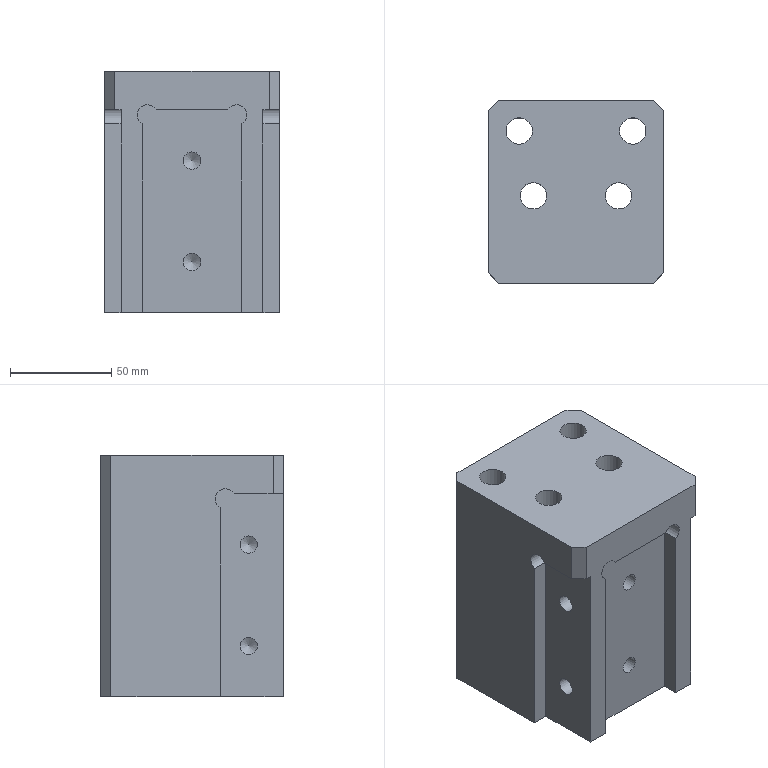Part | NX | features UB-5 2 | 1 solid | 50 faces | box 86 x 90 x 119 mm | volume 701688 mm3 | plane 24 | cylinder 19 | cone 7 | commonest cylinder face diameters 8.5 x6 10 x4 13.007 x4 20 x4 8.506 x1
STEP:
#1=CARTESIAN_POINT('',(3162.594,-722.122,881.466));
#2=VERTEX_POINT('',#1);
#3=CARTESIAN_POINT('',(3162.594,-722.122,885.716));
#4=DIRECTION('',(0.,1.,0.));
#5=DIRECTION('',(0.,0.,-1.));
#6=AXIS2_PLACEMENT_3D('',#3,#4,#5);
#7=CIRCLE('',#6,4.25);
#8=EDGE_CURVE('',#2,#2,#7,.T.);
#9=ORIENTED_EDGE('',*,*,#8,.F.);
#10=EDGE_LOOP('',(#9));
#11=FACE_BOUND('',#10,.T.);
#12=CARTESIAN_POINT('',(3162.594,-719.568,885.716));
#13=VERTEX_POINT('',#12);
#14=VERTEX_LOOP('',#13);
#15=FACE_BOUND('',#14,.T.);
#16=CARTESIAN_POINT('',(3162.594,-722.122,885.716));
#17=DIRECTION('',(0.,-1.,0.));
#18=DIRECTION('',(0.,0.,1.));
#19=AXIS2_PLACEMENT_3D('',#16,#17,#18);
#20=CONICAL_SURFACE('',#19,4.25,1.03);
#21=ADVANCED_FACE('',(#11,#15),#20,.F.);
#22=CARTESIAN_POINT('',(3162.594,-722.122,931.466));
#23=VERTEX_POINT('',#22);
#24=CARTESIAN_POINT('',(3162.594,-722.122,935.716));
#25=DIRECTION('',(0.,1.,0.));
#26=DIRECTION('',(0.,0.,-1.));
#27=AXIS2_PLACEMENT_3D('',#24,#25,#26);
#28=CIRCLE('',#27,4.25);
#29=EDGE_CURVE('',#23,#23,#28,.T.);
#30=ORIENTED_EDGE('',*,*,#29,.F.);
#31=EDGE_LOOP('',(#30));
#32=FACE_BOUND('',#31,.T.);
#33=CARTESIAN_POINT('',(3162.594,-719.568,935.716));
#34=VERTEX_POINT('',#33);
#35=VERTEX_LOOP('',#34);
#36=FACE_BOUND('',#35,.T.);
#37=CARTESIAN_POINT('',(3162.594,-722.122,935.716));
#38=DIRECTION('',(0.,-1.,0.));
#39=DIRECTION('',(0.,0.,1.));
#40=AXIS2_PLACEMENT_3D('',#37,#38,#39);
#41=CONICAL_SURFACE('',#40,4.25,1.03);
#42=ADVANCED_FACE('',(#32,#36),#41,.F.);
#43=CARTESIAN_POINT('',(3147.594,-733.122,881.466));
#44=VERTEX_POINT('',#43);
#45=CARTESIAN_POINT('',(3147.594,-733.122,885.716));
#46=DIRECTION('',(1.,0.,0.));
#47=DIRECTION('',(0.,0.,-1.));
#48=AXIS2_PLACEMENT_3D('',#45,#46,#47);
#49=CIRCLE('',#48,4.25);
#50=EDGE_CURVE('',#44,#44,#49,.T.);
#51=ORIENTED_EDGE('',*,*,#50,.F.);
#52=EDGE_LOOP('',(#51));
#53=FACE_BOUND('',#52,.T.);
#54=CARTESIAN_POINT('',(3150.148,-733.122,885.716));
#55=VERTEX_POINT('',#54);
#56=VERTEX_LOOP('',#55);
#57=FACE_BOUND('',#56,.T.);
#58=CARTESIAN_POINT('',(3147.594,-733.122,885.716));
#59=DIRECTION('',(-1.,0.,0.));
#60=DIRECTION('',(0.,0.,1.));
#61=AXIS2_PLACEMENT_3D('',#58,#59,#60);
#62=CONICAL_SURFACE('',#61,4.25,1.03);
#63=ADVANCED_FACE('',(#53,#57),#62,.F.);
#64=CARTESIAN_POINT('',(3147.594,-733.122,931.466));
#65=VERTEX_POINT('',#64);
#66=CARTESIAN_POINT('',(3147.594,-733.122,935.716));
#67=DIRECTION('',(1.,0.,0.));
#68=DIRECTION('',(0.,0.,-1.));
#69=AXIS2_PLACEMENT_3D('',#66,#67,#68);
#70=CIRCLE('',#69,4.25);
#71=EDGE_CURVE('',#65,#65,#70,.T.);
#72=ORIENTED_EDGE('',*,*,#71,.F.);
#73=EDGE_LOOP('',(#72));
#74=FACE_BOUND('',#73,.T.);
#75=CARTESIAN_POINT('',(3150.148,-733.122,935.716));
#76=VERTEX_POINT('',#75);
#77=VERTEX_LOOP('',#76);
#78=FACE_BOUND('',#77,.T.);
#79=CARTESIAN_POINT('',(3147.594,-733.122,935.716));
#80=DIRECTION('',(-1.,0.,0.));
#81=DIRECTION('',(0.,0.,1.));
#82=AXIS2_PLACEMENT_3D('',#79,#80,#81);
#83=CONICAL_SURFACE('',#82,4.25,1.03);
#84=ADVANCED_FACE('',(#74,#78),#83,.F.);
#85=CARTESIAN_POINT('',(3177.594,-733.122,889.966));
#86=VERTEX_POINT('',#85);
#87=CARTESIAN_POINT('',(3177.594,-733.122,885.716));
#88=DIRECTION('',(-1.,0.,0.));
#89=DIRECTION('',(0.,0.,1.));
#90=AXIS2_PLACEMENT_3D('',#87,#88,#89);
#91=CIRCLE('',#90,4.25);
#92=EDGE_CURVE('',#86,#86,#91,.T.);
#93=ORIENTED_EDGE('',*,*,#92,.F.);
#94=EDGE_LOOP('',(#93));
#95=FACE_BOUND('',#94,.T.);
#96=CARTESIAN_POINT('',(3175.04,-733.122,885.716));
#97=VERTEX_POINT('',#96);
#98=VERTEX_LOOP('',#97);
#99=FACE_BOUND('',#98,.T.);
#100=CARTESIAN_POINT('',(3177.594,-733.122,885.716));
#101=DIRECTION('',(1.,0.,0.));
#102=DIRECTION('',(0.,0.,-1.));
#103=AXIS2_PLACEMENT_3D('',#100,#101,#102);
#104=CONICAL_SURFACE('',#103,4.25,1.03);
#105=ADVANCED_FACE('',(#95,#99),#104,.F.);
#106=CARTESIAN_POINT('',(3177.594,-733.122,939.966));
#107=VERTEX_POINT('',#106);
#108=CARTESIAN_POINT('',(3177.594,-733.122,935.716));
#109=DIRECTION('',(-1.,0.,0.));
#110=DIRECTION('',(0.,0.,1.));
#111=AXIS2_PLACEMENT_3D('',#108,#109,#110);
#112=CIRCLE('',#111,4.25);
#113=EDGE_CURVE('',#107,#107,#112,.T.);
#114=ORIENTED_EDGE('',*,*,#113,.F.);
#115=EDGE_LOOP('',(#114));
#116=FACE_BOUND('',#115,.T.);
#117=CARTESIAN_POINT('',(3175.04,-733.122,935.716));
#118=VERTEX_POINT('',#117);
#119=VERTEX_LOOP('',#118);
#120=FACE_BOUND('',#119,.T.);
#121=CARTESIAN_POINT('',(3177.594,-733.122,935.716));
#122=DIRECTION('',(1.,0.,0.));
#123=DIRECTION('',(0.,0.,-1.));
#124=AXIS2_PLACEMENT_3D('',#121,#122,#123);
#125=CONICAL_SURFACE('',#124,4.25,1.03);
#126=ADVANCED_FACE('',(#116,#120),#125,.F.);
#127=ORIENTED_EDGE('',*,*,#8,.T.);
#128=EDGE_LOOP('',(#127));
#129=FACE_BOUND('',#128,.T.);
#130=CARTESIAN_POINT('',(3162.594,-742.122,881.466));
#131=VERTEX_POINT('',#130);
#132=CARTESIAN_POINT('',(3162.594,-742.122,885.716));
#133=DIRECTION('',(0.,-1.,0.));
#134=DIRECTION('',(0.,0.,-1.));
#135=AXIS2_PLACEMENT_3D('',#132,#133,#134);
#136=CIRCLE('',#135,4.25);
#137=EDGE_CURVE('',#131,#131,#136,.T.);
#138=ORIENTED_EDGE('',*,*,#137,.T.);
#139=EDGE_LOOP('',(#138));
#140=FACE_BOUND('',#139,.T.);
#141=CARTESIAN_POINT('',(3162.594,-742.122,885.716));
#142=DIRECTION('',(0.,1.,0.));
#143=DIRECTION('',(0.,0.,-1.));
#144=AXIS2_PLACEMENT_3D('',#141,#142,#143);
#145=CYLINDRICAL_SURFACE('',#144,4.25);
#146=ADVANCED_FACE('',(#129,#140),#145,.F.);
#147=ORIENTED_EDGE('',*,*,#29,.T.);
#148=EDGE_LOOP('',(#147));
#149=FACE_BOUND('',#148,.T.);
#150=CARTESIAN_POINT('',(3162.594,-742.122,931.466));
#151=VERTEX_POINT('',#150);
#152=CARTESIAN_POINT('',(3162.594,-742.122,935.716));
#153=DIRECTION('',(0.,-1.,0.));
#154=DIRECTION('',(0.,0.,-1.));
#155=AXIS2_PLACEMENT_3D('',#152,#153,#154);
#156=CIRCLE('',#155,4.25);
#157=EDGE_CURVE('',#151,#151,#156,.T.);
#158=ORIENTED_EDGE('',*,*,#157,.T.);
#159=EDGE_LOOP('',(#158));
#160=FACE_BOUND('',#159,.T.);
#161=CARTESIAN_POINT('',(3162.594,-742.122,935.716));
#162=DIRECTION('',(0.,1.,0.));
#163=DIRECTION('',(0.,0.,-1.));
#164=AXIS2_PLACEMENT_3D('',#161,#162,#163);
#165=CYLINDRICAL_SURFACE('',#164,4.25);
#166=ADVANCED_FACE('',(#149,#160),#165,.F.);
#167=CARTESIAN_POINT('',(3138.094,-742.122,953.886));
#168=VERTEX_POINT('',#167);
#169=CARTESIAN_POINT('',(3144.924,-742.122,960.716));
#170=VERTEX_POINT('',#169);
#171=CARTESIAN_POINT('',(3140.594,-742.122,958.216));
#172=DIRECTION('',(0.,1.,0.));
#173=DIRECTION('',(0.,0.,-1.));
#174=AXIS2_PLACEMENT_3D('',#171,#172,#173);
#175=CIRCLE('',#174,5.);
#176=EDGE_CURVE('',#168,#170,#175,.T.);
#177=ORIENTED_EDGE('',*,*,#176,.T.);
#178=CARTESIAN_POINT('',(3144.924,-750.122,960.716));
#179=VERTEX_POINT('',#178);
#180=CARTESIAN_POINT('',(3144.924,-746.122,960.716));
#181=DIRECTION('',(0.,-1.,0.));
#182=VECTOR('',#181,1000.);
#183=LINE('',#180,#182);
#184=EDGE_CURVE('',#170,#179,#183,.T.);
#185=ORIENTED_EDGE('',*,*,#184,.T.);
#186=CARTESIAN_POINT('',(3138.094,-750.122,953.886));
#187=VERTEX_POINT('',#186);
#188=CARTESIAN_POINT('',(3140.594,-750.122,958.216));
#189=DIRECTION('',(0.,-1.,0.));
#190=DIRECTION('',(0.,0.,-1.));
#191=AXIS2_PLACEMENT_3D('',#188,#189,#190);
#192=CIRCLE('',#191,5.);
#193=EDGE_CURVE('',#179,#187,#192,.T.);
#194=ORIENTED_EDGE('',*,*,#193,.T.);
#195=CARTESIAN_POINT('',(3138.094,-750.122,953.886));
#196=DIRECTION('',(0.,1.,0.));
#197=VECTOR('',#196,1000.);
#198=LINE('',#195,#197);
#199=EDGE_CURVE('',#187,#168,#198,.T.);
#200=ORIENTED_EDGE('',*,*,#199,.T.);
#201=EDGE_LOOP('',(#177,#185,#194,#200));
#202=FACE_BOUND('',#201,.T.);
#203=CARTESIAN_POINT('',(3140.594,-750.122,958.216));
#204=DIRECTION('',(0.,1.,0.));
#205=DIRECTION('',(0.,0.,-1.));
#206=AXIS2_PLACEMENT_3D('',#203,#204,#205);
#207=CYLINDRICAL_SURFACE('',#206,5.);
#208=ADVANCED_FACE('',(#202),#207,.F.);
#209=CARTESIAN_POINT('',(3180.264,-750.122,960.716));
#210=VERTEX_POINT('',#209);
#211=CARTESIAN_POINT('',(3162.594,-750.122,960.716));
#212=DIRECTION('',(1.,0.,0.));
#213=VECTOR('',#212,1000.);
#214=LINE('',#211,#213);
#215=EDGE_CURVE('',#179,#210,#214,.T.);
#216=ORIENTED_EDGE('',*,*,#215,.F.);
#217=ORIENTED_EDGE('',*,*,#184,.F.);
#218=CARTESIAN_POINT('',(3180.264,-742.122,960.716));
#219=VERTEX_POINT('',#218);
#220=CARTESIAN_POINT('',(3162.594,-742.122,960.716));
#221=DIRECTION('',(1.,0.,0.));
#222=VECTOR('',#221,1000.);
#223=LINE('',#220,#222);
#224=EDGE_CURVE('',#170,#219,#223,.T.);
#225=ORIENTED_EDGE('',*,*,#224,.T.);
#226=CARTESIAN_POINT('',(3180.264,-746.122,960.716));
#227=DIRECTION('',(0.,1.,0.));
#228=VECTOR('',#227,1000.);
#229=LINE('',#226,#228);
#230=EDGE_CURVE('',#210,#219,#229,.T.);
#231=ORIENTED_EDGE('',*,*,#230,.F.);
#232=EDGE_LOOP('',(#216,#217,#225,#231));
#233=FACE_BOUND('',#232,.T.);
#234=CARTESIAN_POINT('',(3162.594,-747.122,960.716));
#235=DIRECTION('',(0.,0.,1.));
#236=DIRECTION('',(1.,0.,0.));
#237=AXIS2_PLACEMENT_3D('',#234,#235,#236);
#238=PLANE('',#237);
#239=ADVANCED_FACE('',(#233),#238,.F.);
#240=CARTESIAN_POINT('',(3187.094,-742.122,953.886));
#241=VERTEX_POINT('',#240);
#242=CARTESIAN_POINT('',(3184.594,-742.122,958.216));
#243=DIRECTION('',(0.,1.,0.));
#244=DIRECTION('',(0.,0.,-1.));
#245=AXIS2_PLACEMENT_3D('',#242,#243,#244);
#246=CIRCLE('',#245,5.);
#247=EDGE_CURVE('',#219,#241,#246,.T.);
#248=ORIENTED_EDGE('',*,*,#247,.T.);
#249=CARTESIAN_POINT('',(3187.094,-750.122,953.886));
#250=VERTEX_POINT('',#249);
#251=CARTESIAN_POINT('',(3187.094,-742.122,953.886));
#252=DIRECTION('',(0.,-1.,0.));
#253=VECTOR('',#252,1000.);
#254=LINE('',#251,#253);
#255=EDGE_CURVE('',#241,#250,#254,.T.);
#256=ORIENTED_EDGE('',*,*,#255,.T.);
#257=CARTESIAN_POINT('',(3184.594,-750.122,958.216));
#258=DIRECTION('',(0.,-1.,0.));
#259=DIRECTION('',(0.,0.,-1.));
#260=AXIS2_PLACEMENT_3D('',#257,#258,#259);
#261=CIRCLE('',#260,5.);
#262=EDGE_CURVE('',#250,#210,#261,.T.);
#263=ORIENTED_EDGE('',*,*,#262,.T.);
#264=ORIENTED_EDGE('',*,*,#230,.T.);
#265=EDGE_LOOP('',(#248,#256,#263,#264));
#266=FACE_BOUND('',#265,.T.);
#267=CARTESIAN_POINT('',(3184.594,-750.122,958.216));
#268=DIRECTION('',(0.,1.,0.));
#269=DIRECTION('',(0.,0.,-1.));
#270=AXIS2_PLACEMENT_3D('',#267,#268,#269);
#271=CYLINDRICAL_SURFACE('',#270,5.);
#272=ADVANCED_FACE('',(#266),#271,.F.);
#273=ORIENTED_EDGE('',*,*,#50,.T.);
#274=EDGE_LOOP('',(#273));
#275=FACE_BOUND('',#274,.T.);
#276=CARTESIAN_POINT('',(3127.594,-733.122,881.466));
#277=VERTEX_POINT('',#276);
#278=CARTESIAN_POINT('',(3127.594,-733.122,885.716));
#279=DIRECTION('',(-1.,0.,0.));
#280=DIRECTION('',(0.,0.,-1.));
#281=AXIS2_PLACEMENT_3D('',#278,#279,#280);
#282=CIRCLE('',#281,4.25);
#283=EDGE_CURVE('',#277,#277,#282,.T.);
#284=ORIENTED_EDGE('',*,*,#283,.T.);
#285=EDGE_LOOP('',(#284));
#286=FACE_BOUND('',#285,.T.);
#287=CARTESIAN_POINT('',(3127.594,-733.122,885.716));
#288=DIRECTION('',(1.,0.,0.));
#289=DIRECTION('',(0.,0.,-1.));
#290=AXIS2_PLACEMENT_3D('',#287,#288,#289);
#291=CYLINDRICAL_SURFACE('',#290,4.25);
#292=ADVANCED_FACE('',(#275,#286),#291,.F.);
#293=ORIENTED_EDGE('',*,*,#71,.T.);
#294=EDGE_LOOP('',(#293));
#295=FACE_BOUND('',#294,.T.);
#296=CARTESIAN_POINT('',(3127.594,-733.122,931.466));
#297=VERTEX_POINT('',#296);
#298=CARTESIAN_POINT('',(3127.594,-733.122,935.716));
#299=DIRECTION('',(-1.,0.,0.));
#300=DIRECTION('',(0.,0.,-1.));
#301=AXIS2_PLACEMENT_3D('',#298,#299,#300);
#302=CIRCLE('',#301,4.25);
#303=EDGE_CURVE('',#297,#297,#302,.T.);
#304=ORIENTED_EDGE('',*,*,#303,.T.);
#305=EDGE_LOOP('',(#304));
#306=FACE_BOUND('',#305,.T.);
#307=CARTESIAN_POINT('',(3127.594,-733.122,935.716));
#308=DIRECTION('',(1.,0.,0.));
#309=DIRECTION('',(0.,0.,-1.));
#310=AXIS2_PLACEMENT_3D('',#307,#308,#309);
#311=CYLINDRICAL_SURFACE('',#310,4.25);
#312=ADVANCED_FACE('',(#295,#306),#311,.F.);
#313=CARTESIAN_POINT('',(3127.594,-725.952,960.716));
#314=VERTEX_POINT('',#313);
#315=CARTESIAN_POINT('',(3119.594,-725.952,960.716));
#316=VERTEX_POINT('',#315);
#317=CARTESIAN_POINT('',(3127.594,-725.952,960.716));
#318=DIRECTION('',(-1.,0.,0.000000001));
#319=VECTOR('',#318,1000.);
#320=LINE('',#317,#319);
#321=EDGE_CURVE('',#314,#316,#320,.T.);
#322=ORIENTED_EDGE('',*,*,#321,.T.);
#323=CARTESIAN_POINT('',(3119.594,-719.122,953.886));
#324=VERTEX_POINT('',#323);
#325=CARTESIAN_POINT('',(3119.594,-721.622,958.216));
#326=DIRECTION('',(-1.,0.,0.));
#327=DIRECTION('',(0.,0.,-1.));
#328=AXIS2_PLACEMENT_3D('',#325,#326,#327);
#329=CIRCLE('',#328,5.);
#330=EDGE_CURVE('',#316,#324,#329,.T.);
#331=ORIENTED_EDGE('',*,*,#330,.T.);
#332=CARTESIAN_POINT('',(3127.594,-719.122,953.886));
#333=VERTEX_POINT('',#332);
#334=CARTESIAN_POINT('',(3127.594,-719.122,953.886));
#335=DIRECTION('',(-1.,0.,0.000000001));
#336=VECTOR('',#335,1000.);
#337=LINE('',#334,#336);
#338=EDGE_CURVE('',#333,#324,#337,.T.);
#339=ORIENTED_EDGE('',*,*,#338,.F.);
#340=CARTESIAN_POINT('',(3127.594,-721.622,958.216));
#341=DIRECTION('',(-1.,0.,0.000000001));
#342=DIRECTION('',(0.000000001,0.,1.));
#343=AXIS2_PLACEMENT_3D('',#340,#341,#342);
#344=CIRCLE('',#343,5.);
#345=EDGE_CURVE('',#314,#333,#344,.T.);
#346=ORIENTED_EDGE('',*,*,#345,.F.);
#347=EDGE_LOOP('',(#322,#331,#339,#346));
#348=FACE_BOUND('',#347,.T.);
#349=CARTESIAN_POINT('',(3127.594,-721.622,958.216));
#350=DIRECTION('',(1.,0.,-0.000000001));
#351=DIRECTION('',(0.000000001,0.,1.));
#352=AXIS2_PLACEMENT_3D('',#349,#350,#351);
#353=CYLINDRICAL_SURFACE('',#352,5.);
#354=ADVANCED_FACE('',(#348),#353,.F.);
#355=CARTESIAN_POINT('',(3127.594,-750.122,960.716));
#356=VERTEX_POINT('',#355);
#357=CARTESIAN_POINT('',(3127.594,-733.122,960.716));
#358=DIRECTION('',(0.,-1.,0.));
#359=VECTOR('',#358,1000.);
#360=LINE('',#357,#359);
#361=EDGE_CURVE('',#314,#356,#360,.T.);
#362=ORIENTED_EDGE('',*,*,#361,.T.);
#363=CARTESIAN_POINT('',(3124.594,-750.122,960.716));
#364=VERTEX_POINT('',#363);
#365=CARTESIAN_POINT('',(3122.594,-750.122,960.716));
#366=DIRECTION('',(-1.,0.,0.));
#367=VECTOR('',#366,1000.);
#368=LINE('',#365,#367);
#369=EDGE_CURVE('',#356,#364,#368,.T.);
#370=ORIENTED_EDGE('',*,*,#369,.T.);
#371=CARTESIAN_POINT('',(3119.594,-745.122,960.716));
#372=VERTEX_POINT('',#371);
#373=CARTESIAN_POINT('',(3119.594,-745.122,960.716));
#374=DIRECTION('',(0.7071,-0.7071,0.));
#375=VECTOR('',#374,1000.);
#376=LINE('',#373,#375);
#377=EDGE_CURVE('',#372,#364,#376,.T.);
#378=ORIENTED_EDGE('',*,*,#377,.F.);
#379=CARTESIAN_POINT('',(3119.594,-722.122,960.716));
#380=DIRECTION('',(0.,1.,0.));
#381=VECTOR('',#380,1000.);
#382=LINE('',#379,#381);
#383=EDGE_CURVE('',#372,#316,#382,.T.);
#384=ORIENTED_EDGE('',*,*,#383,.T.);
#385=ORIENTED_EDGE('',*,*,#321,.F.);
#386=EDGE_LOOP('',(#362,#370,#378,#384,#385));
#387=FACE_BOUND('',#386,.T.);
#388=CARTESIAN_POINT('',(3122.594,-733.122,960.716));
#389=DIRECTION('',(0.,0.,1.));
#390=DIRECTION('',(1.,0.,0.));
#391=AXIS2_PLACEMENT_3D('',#388,#389,#390);
#392=PLANE('',#391);
#393=ADVANCED_FACE('',(#387),#392,.F.);
#394=CARTESIAN_POINT('',(3197.594,-725.952,960.716));
#395=VERTEX_POINT('',#394);
#396=CARTESIAN_POINT('',(3197.594,-719.122,953.886));
#397=VERTEX_POINT('',#396);
#398=CARTESIAN_POINT('',(3197.594,-721.622,958.216));
#399=DIRECTION('',(-1.,0.,0.));
#400=DIRECTION('',(0.,0.,1.));
#401=AXIS2_PLACEMENT_3D('',#398,#399,#400);
#402=CIRCLE('',#401,5.);
#403=EDGE_CURVE('',#395,#397,#402,.T.);
#404=ORIENTED_EDGE('',*,*,#403,.T.);
#405=CARTESIAN_POINT('',(3205.594,-719.122,953.886));
#406=VERTEX_POINT('',#405);
#407=CARTESIAN_POINT('',(3201.594,-719.122,953.886));
#408=DIRECTION('',(1.,0.,0.));
#409=VECTOR('',#408,1000.);
#410=LINE('',#407,#409);
#411=EDGE_CURVE('',#397,#406,#410,.T.);
#412=ORIENTED_EDGE('',*,*,#411,.T.);
#413=CARTESIAN_POINT('',(3205.594,-725.952,960.716));
#414=VERTEX_POINT('',#413);
#415=CARTESIAN_POINT('',(3205.594,-721.622,958.216));
#416=DIRECTION('',(1.,0.,0.));
#417=DIRECTION('',(0.,0.,-1.));
#418=AXIS2_PLACEMENT_3D('',#415,#416,#417);
#419=CIRCLE('',#418,5.);
#420=EDGE_CURVE('',#406,#414,#419,.T.);
#421=ORIENTED_EDGE('',*,*,#420,.T.);
#422=CARTESIAN_POINT('',(3201.594,-725.952,960.716));
#423=DIRECTION('',(-1.,0.,0.));
#424=VECTOR('',#423,1000.);
#425=LINE('',#422,#424);
#426=EDGE_CURVE('',#414,#395,#425,.T.);
#427=ORIENTED_EDGE('',*,*,#426,.T.);
#428=EDGE_LOOP('',(#404,#412,#421,#427));
#429=FACE_BOUND('',#428,.T.);
#430=CARTESIAN_POINT('',(3205.594,-721.622,958.216));
#431=DIRECTION('',(-1.,0.,0.));
#432=DIRECTION('',(0.,0.,1.));
#433=AXIS2_PLACEMENT_3D('',#430,#431,#432);
#434=CYLINDRICAL_SURFACE('',#433,5.);
#435=ADVANCED_FACE('',(#429),#434,.F.);
#436=CARTESIAN_POINT('',(3205.594,-745.122,960.716));
#437=VERTEX_POINT('',#436);
#438=CARTESIAN_POINT('',(3205.594,-722.122,960.716));
#439=DIRECTION('',(0.,1.,0.));
#440=VECTOR('',#439,1000.);
#441=LINE('',#438,#440);
#442=EDGE_CURVE('',#437,#414,#441,.T.);
#443=ORIENTED_EDGE('',*,*,#442,.F.);
#444=CARTESIAN_POINT('',(3200.594,-750.122,960.716));
#445=VERTEX_POINT('',#444);
#446=CARTESIAN_POINT('',(3200.594,-750.122,960.716));
#447=DIRECTION('',(0.7071,0.7071,0.));
#448=VECTOR('',#447,1000.);
#449=LINE('',#446,#448);
#450=EDGE_CURVE('',#445,#437,#449,.T.);
#451=ORIENTED_EDGE('',*,*,#450,.F.);
#452=CARTESIAN_POINT('',(3197.594,-750.122,960.716));
#453=VERTEX_POINT('',#452);
#454=CARTESIAN_POINT('',(3202.594,-750.122,960.716));
#455=DIRECTION('',(-1.,0.,0.));
#456=VECTOR('',#455,1000.);
#457=LINE('',#454,#456);
#458=EDGE_CURVE('',#445,#453,#457,.T.);
#459=ORIENTED_EDGE('',*,*,#458,.T.);
#460=CARTESIAN_POINT('',(3197.594,-733.122,960.716));
#461=DIRECTION('',(0.,1.,0.));
#462=VECTOR('',#461,1000.);
#463=LINE('',#460,#462);
#464=EDGE_CURVE('',#453,#395,#463,.T.);
#465=ORIENTED_EDGE('',*,*,#464,.T.);
#466=ORIENTED_EDGE('',*,*,#426,.F.);
#467=EDGE_LOOP('',(#443,#451,#459,#465,#466));
#468=FACE_BOUND('',#467,.T.);
#469=CARTESIAN_POINT('',(3202.594,-733.122,960.716));
#470=DIRECTION('',(0.,0.,1.));
#471=DIRECTION('',(1.,0.,0.));
#472=AXIS2_PLACEMENT_3D('',#469,#470,#471);
#473=PLANE('',#472);
#474=ADVANCED_FACE('',(#468),#473,.F.);
#475=ORIENTED_EDGE('',*,*,#92,.T.);
#476=EDGE_LOOP('',(#475));
#477=FACE_BOUND('',#476,.T.);
#478=CARTESIAN_POINT('',(3197.594,-733.122,889.966));
#479=VERTEX_POINT('',#478);
#480=CARTESIAN_POINT('',(3197.594,-733.122,885.716));
#481=DIRECTION('',(1.,0.,0.));
#482=DIRECTION('',(0.,0.,1.));
#483=AXIS2_PLACEMENT_3D('',#480,#481,#482);
#484=CIRCLE('',#483,4.25);
#485=EDGE_CURVE('',#479,#479,#484,.T.);
#486=ORIENTED_EDGE('',*,*,#485,.T.);
#487=EDGE_LOOP('',(#486));
#488=FACE_BOUND('',#487,.T.);
#489=CARTESIAN_POINT('',(3197.594,-733.122,885.716));
#490=DIRECTION('',(-1.,0.,0.));
#491=DIRECTION('',(0.,0.,1.));
#492=AXIS2_PLACEMENT_3D('',#489,#490,#491);
#493=CYLINDRICAL_SURFACE('',#492,4.25);
#494=ADVANCED_FACE('',(#477,#488),#493,.F.);
#495=ORIENTED_EDGE('',*,*,#113,.T.);
#496=EDGE_LOOP('',(#495));
#497=FACE_BOUND('',#496,.T.);
#498=CARTESIAN_POINT('',(3197.594,-733.122,939.966));
#499=VERTEX_POINT('',#498);
#500=CARTESIAN_POINT('',(3197.594,-733.122,935.716));
#501=DIRECTION('',(1.,0.,0.));
#502=DIRECTION('',(0.,0.,1.));
#503=AXIS2_PLACEMENT_3D('',#500,#501,#502);
#504=CIRCLE('',#503,4.25);
#505=EDGE_CURVE('',#499,#499,#504,.T.);
#506=ORIENTED_EDGE('',*,*,#505,.T.);
#507=EDGE_LOOP('',(#506));
#508=FACE_BOUND('',#507,.T.);
#509=CARTESIAN_POINT('',(3197.594,-733.122,935.716));
#510=DIRECTION('',(-1.,0.,0.));
#511=DIRECTION('',(0.,0.,1.));
#512=AXIS2_PLACEMENT_3D('',#509,#510,#511);
#513=CYLINDRICAL_SURFACE('',#512,4.25);
#514=ADVANCED_FACE('',(#497,#508),#513,.F.);
#515=CARTESIAN_POINT('',(3148.097,-707.122,935.716));
#516=VERTEX_POINT('',#515);
#517=CARTESIAN_POINT('',(3141.594,-707.122,935.716));
#518=DIRECTION('',(0.,0.,1.));
#519=DIRECTION('',(1.,0.,0.));
#520=AXIS2_PLACEMENT_3D('',#517,#518,#519);
#521=CIRCLE('',#520,6.503);
#522=EDGE_CURVE('',#516,#516,#521,.T.);
#523=ORIENTED_EDGE('',*,*,#522,.T.);
#524=EDGE_LOOP('',(#523));
#525=FACE_BOUND('',#524,.T.);
#526=CARTESIAN_POINT('',(3151.594,-707.122,935.716));
#527=VERTEX_POINT('',#526);
#528=CARTESIAN_POINT('',(3141.594,-707.122,935.716));
#529=DIRECTION('',(0.,0.,1.));
#530=DIRECTION('',(1.,0.,0.));
#531=AXIS2_PLACEMENT_3D('',#528,#529,#530);
#532=CIRCLE('',#531,10.);
#533=EDGE_CURVE('',#527,#527,#532,.T.);
#534=ORIENTED_EDGE('',*,*,#533,.F.);
#535=EDGE_LOOP('',(#534));
#536=FACE_BOUND('',#535,.T.);
#537=CARTESIAN_POINT('',(3141.594,-707.122,935.716));
#538=DIRECTION('',(0.,0.,1.));
#539=DIRECTION('',(1.,0.,0.));
#540=AXIS2_PLACEMENT_3D('',#537,#538,#539);
#541=PLANE('',#540);
#542=ADVANCED_FACE('',(#525,#536),#541,.F.);
#543=CARTESIAN_POINT('',(3190.097,-707.122,935.716));
#544=VERTEX_POINT('',#543);
#545=CARTESIAN_POINT('',(3183.594,-707.122,935.716));
#546=DIRECTION('',(0.,0.,1.));
#547=DIRECTION('',(1.,0.,0.));
#548=AXIS2_PLACEMENT_3D('',#545,#546,#547);
#549=CIRCLE('',#548,6.503);
#550=EDGE_CURVE('',#544,#544,#549,.T.);
#551=ORIENTED_EDGE('',*,*,#550,.T.);
#552=EDGE_LOOP('',(#551));
#553=FACE_BOUND('',#552,.T.);
#554=CARTESIAN_POINT('',(3173.594,-707.122,935.716));
#555=VERTEX_POINT('',#554);
#556=CARTESIAN_POINT('',(3183.594,-707.122,935.716));
#557=DIRECTION('',(0.,0.,1.));
#558=DIRECTION('',(-1.,0.,0.));
#559=AXIS2_PLACEMENT_3D('',#556,#557,#558);
#560=CIRCLE('',#559,10.);
#561=EDGE_CURVE('',#555,#555,#560,.T.);
#562=ORIENTED_EDGE('',*,*,#561,.F.);
#563=EDGE_LOOP('',(#562));
#564=FACE_BOUND('',#563,.T.);
#565=CARTESIAN_POINT('',(3183.594,-707.122,935.716));
#566=DIRECTION('',(0.,0.,1.));
#567=DIRECTION('',(-1.,0.,0.));
#568=AXIS2_PLACEMENT_3D('',#565,#566,#567);
#569=PLANE('',#568);
#570=ADVANCED_FACE('',(#553,#564),#569,.F.);
#571=CARTESIAN_POINT('',(3141.097,-675.122,935.716));
#572=VERTEX_POINT('',#571);
#573=CARTESIAN_POINT('',(3134.594,-675.122,935.716));
#574=DIRECTION('',(0.,0.,1.));
#575=DIRECTION('',(1.,0.,0.));
#576=AXIS2_PLACEMENT_3D('',#573,#574,#575);
#577=CIRCLE('',#576,6.503);
#578=EDGE_CURVE('',#572,#572,#577,.T.);
#579=ORIENTED_EDGE('',*,*,#578,.T.);
#580=EDGE_LOOP('',(#579));
#581=FACE_BOUND('',#580,.T.);
#582=CARTESIAN_POINT('',(3144.594,-675.122,935.716));
#583=VERTEX_POINT('',#582);
#584=CARTESIAN_POINT('',(3134.594,-675.122,935.716));
#585=DIRECTION('',(0.,0.,1.));
#586=DIRECTION('',(1.,0.,0.));
#587=AXIS2_PLACEMENT_3D('',#584,#585,#586);
#588=CIRCLE('',#587,10.);
#589=EDGE_CURVE('',#583,#583,#588,.T.);
#590=ORIENTED_EDGE('',*,*,#589,.F.);
#591=EDGE_LOOP('',(#590));
#592=FACE_BOUND('',#591,.T.);
#593=CARTESIAN_POINT('',(3134.594,-675.122,935.716));
#594=DIRECTION('',(0.,0.,1.));
#595=DIRECTION('',(1.,0.,0.));
#596=AXIS2_PLACEMENT_3D('',#593,#594,#595);
#597=PLANE('',#596);
#598=ADVANCED_FACE('',(#581,#592),#597,.F.);
#599=ORIENTED_EDGE('',*,*,#377,.T.);
#600=CARTESIAN_POINT('',(3124.594,-750.122,979.716));
#601=VERTEX_POINT('',#600);
#602=CARTESIAN_POINT('',(3124.594,-750.122,1005.716));
#603=DIRECTION('',(0.,0.,1.));
#604=VECTOR('',#603,1000.);
#605=LINE('',#602,#604);
#606=EDGE_CURVE('',#364,#601,#605,.T.);
#607=ORIENTED_EDGE('',*,*,#606,.T.);
#608=CARTESIAN_POINT('',(3119.594,-745.122,979.716));
#609=VERTEX_POINT('',#608);
#610=CARTESIAN_POINT('',(3560.844,-1186.372,979.716));
#611=DIRECTION('',(-0.7071,0.7071,0.));
#612=VECTOR('',#611,1000.);
#613=LINE('',#610,#612);
#614=EDGE_CURVE('',#601,#609,#613,.T.);
#615=ORIENTED_EDGE('',*,*,#614,.T.);
#616=CARTESIAN_POINT('',(3119.594,-745.122,885.716));
#617=DIRECTION('',(0.,0.,-1.));
#618=VECTOR('',#617,1000.);
#619=LINE('',#616,#618);
#620=EDGE_CURVE('',#609,#372,#619,.T.);
#621=ORIENTED_EDGE('',*,*,#620,.T.);
#622=EDGE_LOOP('',(#599,#607,#615,#621));
#623=FACE_BOUND('',#622,.T.);
#624=CARTESIAN_POINT('',(3119.594,-745.122,915.716));
#625=DIRECTION('',(0.7071,0.7071,0.));
#626=DIRECTION('',(0.,0.,-1.));
#627=AXIS2_PLACEMENT_3D('',#624,#625,#626);
#628=PLANE('',#627);
#629=ADVANCED_FACE('',(#623),#628,.F.);
#630=ORIENTED_EDGE('',*,*,#450,.T.);
#631=CARTESIAN_POINT('',(3205.594,-745.122,979.716));
#632=VERTEX_POINT('',#631);
#633=CARTESIAN_POINT('',(3205.594,-745.122,915.716));
#634=DIRECTION('',(0.,0.,1.));
#635=VECTOR('',#634,1000.);
#636=LINE('',#633,#635);
#637=EDGE_CURVE('',#437,#632,#636,.T.);
#638=ORIENTED_EDGE('',*,*,#637,.T.);
#639=CARTESIAN_POINT('',(3200.594,-750.122,979.716));
#640=VERTEX_POINT('',#639);
#641=CARTESIAN_POINT('',(3200.594,-750.122,979.716));
#642=DIRECTION('',(-0.7071,-0.7071,0.));
#643=VECTOR('',#642,1000.);
#644=LINE('',#641,#643);
#645=EDGE_CURVE('',#632,#640,#644,.T.);
#646=ORIENTED_EDGE('',*,*,#645,.T.);
#647=CARTESIAN_POINT('',(3200.594,-750.122,864.216));
#648=DIRECTION('',(0.,0.,-1.));
#649=VECTOR('',#648,1000.);
#650=LINE('',#647,#649);
#651=EDGE_CURVE('',#640,#445,#650,.T.);
#652=ORIENTED_EDGE('',*,*,#651,.T.);
#653=EDGE_LOOP('',(#630,#638,#646,#652));
#654=FACE_BOUND('',#653,.T.);
#655=CARTESIAN_POINT('',(3200.594,-750.122,864.216));
#656=DIRECTION('',(0.7071,-0.7071,0.));
#657=DIRECTION('',(0.,0.,1.));
#658=AXIS2_PLACEMENT_3D('',#655,#656,#657);
#659=PLANE('',#658);
#660=ADVANCED_FACE('',(#654),#659,.T.);
#661=CARTESIAN_POINT('',(3187.094,-742.122,860.716));
#662=VERTEX_POINT('',#661);
#663=CARTESIAN_POINT('',(3187.094,-742.122,885.716));
#664=DIRECTION('',(0.,0.,-1.));
#665=VECTOR('',#664,1000.);
#666=LINE('',#663,#665);
#667=EDGE_CURVE('',#241,#662,#666,.T.);
#668=ORIENTED_EDGE('',*,*,#667,.T.);
#669=CARTESIAN_POINT('',(3187.094,-750.122,860.716));
#670=VERTEX_POINT('',#669);
#671=CARTESIAN_POINT('',(3187.094,-747.122,860.716));
#672=DIRECTION('',(0.,-1.,0.));
#673=VECTOR('',#672,1000.);
#674=LINE('',#671,#673);
#675=EDGE_CURVE('',#662,#670,#674,.T.);
#676=ORIENTED_EDGE('',*,*,#675,.T.);
#677=CARTESIAN_POINT('',(3187.094,-750.122,864.216));
#678=DIRECTION('',(0.,0.,-1.));
#679=VECTOR('',#678,1000.);
#680=LINE('',#677,#679);
#681=EDGE_CURVE('',#250,#670,#680,.T.);
#682=ORIENTED_EDGE('',*,*,#681,.F.);
#683=ORIENTED_EDGE('',*,*,#255,.F.);
#684=EDGE_LOOP('',(#668,#676,#682,#683));
#685=FACE_BOUND('',#684,.T.);
#686=CARTESIAN_POINT('',(3187.094,-747.122,885.716));
#687=DIRECTION('',(1.,0.,0.));
#688=DIRECTION('',(0.,0.,-1.));
#689=AXIS2_PLACEMENT_3D('',#686,#687,#688);
#690=PLANE('',#689);
#691=ADVANCED_FACE('',(#685),#690,.F.);
#692=ORIENTED_EDGE('',*,*,#157,.F.);
#693=EDGE_LOOP('',(#692));
#694=FACE_BOUND('',#693,.T.);
#695=ORIENTED_EDGE('',*,*,#137,.F.);
#696=EDGE_LOOP('',(#695));
#697=FACE_BOUND('',#696,.T.);
#698=ORIENTED_EDGE('',*,*,#224,.F.);
#699=ORIENTED_EDGE('',*,*,#176,.F.);
#700=CARTESIAN_POINT('',(3138.094,-742.122,860.716));
#701=VERTEX_POINT('',#700);
#702=CARTESIAN_POINT('',(3138.094,-742.122,885.716));
#703=DIRECTION('',(0.,0.,-1.));
#704=VECTOR('',#703,1000.);
#705=LINE('',#702,#704);
#706=EDGE_CURVE('',#168,#701,#705,.T.);
#707=ORIENTED_EDGE('',*,*,#706,.T.);
#708=CARTESIAN_POINT('',(3162.594,-742.122,860.716));
#709=DIRECTION('',(1.,0.,0.));
#710=VECTOR('',#709,1000.);
#711=LINE('',#708,#710);
#712=EDGE_CURVE('',#701,#662,#711,.T.);
#713=ORIENTED_EDGE('',*,*,#712,.T.);
#714=ORIENTED_EDGE('',*,*,#667,.F.);
#715=ORIENTED_EDGE('',*,*,#247,.F.);
#716=EDGE_LOOP('',(#698,#699,#707,#713,#714,#715));
#717=FACE_BOUND('',#716,.T.);
#718=CARTESIAN_POINT('',(3162.594,-742.122,885.716));
#719=DIRECTION('',(0.,1.,0.));
#720=DIRECTION('',(0.,0.,-1.));
#721=AXIS2_PLACEMENT_3D('',#718,#719,#720);
#722=PLANE('',#721);
#723=ADVANCED_FACE('',(#694,#697,#717),#722,.F.);
#724=CARTESIAN_POINT('',(3138.094,-750.122,860.716));
#725=VERTEX_POINT('',#724);
#726=CARTESIAN_POINT('',(3138.094,-750.122,864.216));
#727=DIRECTION('',(0.,0.,1.));
#728=VECTOR('',#727,1000.);
#729=LINE('',#726,#728);
#730=EDGE_CURVE('',#725,#187,#729,.T.);
#731=ORIENTED_EDGE('',*,*,#730,.F.);
#732=CARTESIAN_POINT('',(3138.094,-747.122,860.716));
#733=DIRECTION('',(0.,1.,0.));
#734=VECTOR('',#733,1000.);
#735=LINE('',#732,#734);
#736=EDGE_CURVE('',#725,#701,#735,.T.);
#737=ORIENTED_EDGE('',*,*,#736,.T.);
#738=ORIENTED_EDGE('',*,*,#706,.F.);
#739=ORIENTED_EDGE('',*,*,#199,.F.);
#740=EDGE_LOOP('',(#731,#737,#738,#739));
#741=FACE_BOUND('',#740,.T.);
#742=CARTESIAN_POINT('',(3138.094,-747.122,885.716));
#743=DIRECTION('',(-1.,0.,0.));
#744=DIRECTION('',(0.,0.,1.));
#745=AXIS2_PLACEMENT_3D('',#742,#743,#744);
#746=PLANE('',#745);
#747=ADVANCED_FACE('',(#741),#746,.F.);
#748=ORIENTED_EDGE('',*,*,#262,.F.);
#749=ORIENTED_EDGE('',*,*,#681,.T.);
#750=CARTESIAN_POINT('',(3197.594,-750.122,860.716));
#751=VERTEX_POINT('',#750);
#752=CARTESIAN_POINT('',(3162.594,-750.122,860.716));
#753=DIRECTION('',(1.,0.,0.));
#754=VECTOR('',#753,1000.);
#755=LINE('',#752,#754);
#756=EDGE_CURVE('',#670,#751,#755,.T.);
#757=ORIENTED_EDGE('',*,*,#756,.T.);
#758=CARTESIAN_POINT('',(3197.594,-750.122,885.716));
#759=DIRECTION('',(0.,0.,-1.));
#760=VECTOR('',#759,1000.);
#761=LINE('',#758,#760);
#762=EDGE_CURVE('',#453,#751,#761,.T.);
#763=ORIENTED_EDGE('',*,*,#762,.F.);
#764=ORIENTED_EDGE('',*,*,#458,.F.);
#765=ORIENTED_EDGE('',*,*,#651,.F.);
#766=CARTESIAN_POINT('',(3162.594,-750.122,979.716));
#767=DIRECTION('',(1.,0.,0.));
#768=VECTOR('',#767,1000.);
#769=LINE('',#766,#768);
#770=EDGE_CURVE('',#601,#640,#769,.T.);
#771=ORIENTED_EDGE('',*,*,#770,.F.);
#772=ORIENTED_EDGE('',*,*,#606,.F.);
#773=ORIENTED_EDGE('',*,*,#369,.F.);
#774=CARTESIAN_POINT('',(3127.594,-750.122,860.716));
#775=VERTEX_POINT('',#774);
#776=CARTESIAN_POINT('',(3127.594,-750.122,864.216));
#777=DIRECTION('',(0.,0.,-1.));
#778=VECTOR('',#777,1000.);
#779=LINE('',#776,#778);
#780=EDGE_CURVE('',#356,#775,#779,.T.);
#781=ORIENTED_EDGE('',*,*,#780,.T.);
#782=CARTESIAN_POINT('',(3162.594,-750.122,860.716));
#783=DIRECTION('',(1.,0.,0.));
#784=VECTOR('',#783,1000.);
#785=LINE('',#782,#784);
#786=EDGE_CURVE('',#775,#725,#785,.T.);
#787=ORIENTED_EDGE('',*,*,#786,.T.);
#788=ORIENTED_EDGE('',*,*,#730,.T.);
#789=ORIENTED_EDGE('',*,*,#193,.F.);
#790=ORIENTED_EDGE('',*,*,#215,.T.);
#791=EDGE_LOOP('',(#748,#749,#757,#763,#764,#765,#771,#772,#773,#781,#787,#788,#789,#790));
#792=FACE_BOUND('',#791,.T.);
#793=CARTESIAN_POINT('',(3162.594,-750.122,864.216));
#794=DIRECTION('',(0.,1.,0.));
#795=DIRECTION('',(0.,0.,-1.));
#796=AXIS2_PLACEMENT_3D('',#793,#794,#795);
#797=PLANE('',#796);
#798=ADVANCED_FACE('',(#792),#797,.F.);
#799=CARTESIAN_POINT('',(3127.594,-719.122,860.716));
#800=VERTEX_POINT('',#799);
#801=CARTESIAN_POINT('',(3127.594,-719.122,885.716));
#802=DIRECTION('',(0.,0.,-1.));
#803=VECTOR('',#802,1000.);
#804=LINE('',#801,#803);
#805=EDGE_CURVE('',#333,#800,#804,.T.);
#806=ORIENTED_EDGE('',*,*,#805,.T.);
#807=CARTESIAN_POINT('',(3127.594,-733.122,860.716));
#808=DIRECTION('',(0.,-1.,0.));
#809=VECTOR('',#808,1000.);
#810=LINE('',#807,#809);
#811=EDGE_CURVE('',#800,#775,#810,.T.);
#812=ORIENTED_EDGE('',*,*,#811,.T.);
#813=ORIENTED_EDGE('',*,*,#780,.F.);
#814=ORIENTED_EDGE('',*,*,#361,.F.);
#815=ORIENTED_EDGE('',*,*,#345,.T.);
#816=EDGE_LOOP('',(#806,#812,#813,#814,#815));
#817=FACE_BOUND('',#816,.T.);
#818=ORIENTED_EDGE('',*,*,#303,.F.);
#819=EDGE_LOOP('',(#818));
#820=FACE_BOUND('',#819,.T.);
#821=ORIENTED_EDGE('',*,*,#283,.F.);
#822=EDGE_LOOP('',(#821));
#823=FACE_BOUND('',#822,.T.);
#824=CARTESIAN_POINT('',(3127.594,-733.122,885.716));
#825=DIRECTION('',(1.,0.,0.));
#826=DIRECTION('',(0.,0.,-1.));
#827=AXIS2_PLACEMENT_3D('',#824,#825,#826);
#828=PLANE('',#827);
#829=ADVANCED_FACE('',(#817,#820,#823),#828,.F.);
#830=CARTESIAN_POINT('',(3119.594,-719.122,860.716));
#831=VERTEX_POINT('',#830);
#832=CARTESIAN_POINT('',(3119.594,-719.122,915.716));
#833=DIRECTION('',(0.,0.,-1.));
#834=VECTOR('',#833,1000.);
#835=LINE('',#832,#834);
#836=EDGE_CURVE('',#324,#831,#835,.T.);
#837=ORIENTED_EDGE('',*,*,#836,.T.);
#838=CARTESIAN_POINT('',(3122.594,-719.122,860.716));
#839=DIRECTION('',(1.,0.,0.));
#840=VECTOR('',#839,1000.);
#841=LINE('',#838,#840);
#842=EDGE_CURVE('',#831,#800,#841,.T.);
#843=ORIENTED_EDGE('',*,*,#842,.T.);
#844=ORIENTED_EDGE('',*,*,#805,.F.);
#845=ORIENTED_EDGE('',*,*,#338,.T.);
#846=EDGE_LOOP('',(#837,#843,#844,#845));
#847=FACE_BOUND('',#846,.T.);
#848=CARTESIAN_POINT('',(3122.594,-719.122,885.716));
#849=DIRECTION('',(0.,1.,0.));
#850=DIRECTION('',(0.,0.,-1.));
#851=AXIS2_PLACEMENT_3D('',#848,#849,#850);
#852=PLANE('',#851);
#853=ADVANCED_FACE('',(#847),#852,.F.);
#854=CARTESIAN_POINT('',(3119.594,-665.122,860.716));
#855=VERTEX_POINT('',#854);
#856=CARTESIAN_POINT('',(3119.594,-722.122,860.716));
#857=DIRECTION('',(0.,1.,0.));
#858=VECTOR('',#857,1000.);
#859=LINE('',#856,#858);
#860=EDGE_CURVE('',#831,#855,#859,.T.);
#861=ORIENTED_EDGE('',*,*,#860,.F.);
#862=ORIENTED_EDGE('',*,*,#836,.F.);
#863=ORIENTED_EDGE('',*,*,#330,.F.);
#864=ORIENTED_EDGE('',*,*,#383,.F.);
#865=ORIENTED_EDGE('',*,*,#620,.F.);
#866=CARTESIAN_POINT('',(3119.594,-665.122,979.716));
#867=VERTEX_POINT('',#866);
#868=CARTESIAN_POINT('',(3119.594,-722.122,979.716));
#869=DIRECTION('',(0.,-1.,0.));
#870=VECTOR('',#869,1000.);
#871=LINE('',#868,#870);
#872=EDGE_CURVE('',#867,#609,#871,.T.);
#873=ORIENTED_EDGE('',*,*,#872,.F.);
#874=CARTESIAN_POINT('',(3119.594,-665.122,1005.716));
#875=DIRECTION('',(0.,0.,1.));
#876=VECTOR('',#875,1000.);
#877=LINE('',#874,#876);
#878=EDGE_CURVE('',#855,#867,#877,.T.);
#879=ORIENTED_EDGE('',*,*,#878,.F.);
#880=EDGE_LOOP('',(#861,#862,#863,#864,#865,#873,#879));
#881=FACE_BOUND('',#880,.T.);
#882=CARTESIAN_POINT('',(3119.594,-722.122,915.716));
#883=DIRECTION('',(1.,0.,0.));
#884=DIRECTION('',(0.,0.,-1.));
#885=AXIS2_PLACEMENT_3D('',#882,#883,#884);
#886=PLANE('',#885);
#887=ADVANCED_FACE('',(#881),#886,.F.);
#888=CARTESIAN_POINT('',(3124.594,-660.122,860.716));
#889=VERTEX_POINT('',#888);
#890=CARTESIAN_POINT('',(3200.594,-660.122,860.716));
#891=VERTEX_POINT('',#890);
#892=CARTESIAN_POINT('',(3162.594,-660.122,860.716));
#893=DIRECTION('',(1.,0.,0.));
#894=VECTOR('',#893,1000.);
#895=LINE('',#892,#894);
#896=EDGE_CURVE('',#889,#891,#895,.T.);
#897=ORIENTED_EDGE('',*,*,#896,.F.);
#898=CARTESIAN_POINT('',(3124.594,-660.122,979.716));
#899=VERTEX_POINT('',#898);
#900=CARTESIAN_POINT('',(3124.594,-660.122,885.716));
#901=DIRECTION('',(0.,0.,-1.));
#902=VECTOR('',#901,1000.);
#903=LINE('',#900,#902);
#904=EDGE_CURVE('',#899,#889,#903,.T.);
#905=ORIENTED_EDGE('',*,*,#904,.F.);
#906=CARTESIAN_POINT('',(3200.594,-660.122,979.716));
#907=VERTEX_POINT('',#906);
#908=CARTESIAN_POINT('',(3162.594,-660.122,979.716));
#909=DIRECTION('',(1.,0.,0.));
#910=VECTOR('',#909,1000.);
#911=LINE('',#908,#910);
#912=EDGE_CURVE('',#899,#907,#911,.T.);
#913=ORIENTED_EDGE('',*,*,#912,.T.);
#914=CARTESIAN_POINT('',(3200.594,-660.122,864.216));
#915=DIRECTION('',(0.,0.,1.));
#916=VECTOR('',#915,1000.);
#917=LINE('',#914,#916);
#918=EDGE_CURVE('',#891,#907,#917,.T.);
#919=ORIENTED_EDGE('',*,*,#918,.F.);
#920=EDGE_LOOP('',(#897,#905,#913,#919));
#921=FACE_BOUND('',#920,.T.);
#922=CARTESIAN_POINT('',(3162.594,-660.122,864.216));
#923=DIRECTION('',(0.,1.,0.));
#924=DIRECTION('',(0.,0.,-1.));
#925=AXIS2_PLACEMENT_3D('',#922,#923,#924);
#926=PLANE('',#925);
#927=ADVANCED_FACE('',(#921),#926,.T.);
#928=CARTESIAN_POINT('',(3205.594,-665.122,979.716));
#929=VERTEX_POINT('',#928);
#930=CARTESIAN_POINT('',(3205.594,-722.122,979.716));
#931=DIRECTION('',(0.,-1.,0.));
#932=VECTOR('',#931,1000.);
#933=LINE('',#930,#932);
#934=EDGE_CURVE('',#929,#632,#933,.T.);
#935=ORIENTED_EDGE('',*,*,#934,.T.);
#936=ORIENTED_EDGE('',*,*,#637,.F.);
#937=ORIENTED_EDGE('',*,*,#442,.T.);
#938=ORIENTED_EDGE('',*,*,#420,.F.);
#939=CARTESIAN_POINT('',(3205.594,-719.122,860.716));
#940=VERTEX_POINT('',#939);
#941=CARTESIAN_POINT('',(3205.594,-719.122,915.716));
#942=DIRECTION('',(0.,0.,-1.));
#943=VECTOR('',#942,1000.);
#944=LINE('',#941,#943);
#945=EDGE_CURVE('',#406,#940,#944,.T.);
#946=ORIENTED_EDGE('',*,*,#945,.T.);
#947=CARTESIAN_POINT('',(3205.594,-665.122,860.716));
#948=VERTEX_POINT('',#947);
#949=CARTESIAN_POINT('',(3205.594,-722.122,860.716));
#950=DIRECTION('',(0.,1.,0.));
#951=VECTOR('',#950,1000.);
#952=LINE('',#949,#951);
#953=EDGE_CURVE('',#940,#948,#952,.T.);
#954=ORIENTED_EDGE('',*,*,#953,.T.);
#955=CARTESIAN_POINT('',(3205.594,-665.122,915.716));
#956=DIRECTION('',(0.,0.,-1.));
#957=VECTOR('',#956,1000.);
#958=LINE('',#955,#957);
#959=EDGE_CURVE('',#929,#948,#958,.T.);
#960=ORIENTED_EDGE('',*,*,#959,.F.);
#961=EDGE_LOOP('',(#935,#936,#937,#938,#946,#954,#960));
#962=FACE_BOUND('',#961,.T.);
#963=CARTESIAN_POINT('',(3205.594,-722.122,915.716));
#964=DIRECTION('',(1.,0.,0.));
#965=DIRECTION('',(0.,0.,-1.));
#966=AXIS2_PLACEMENT_3D('',#963,#964,#965);
#967=PLANE('',#966);
#968=ADVANCED_FACE('',(#962),#967,.T.);
#969=CARTESIAN_POINT('',(3197.594,-719.122,860.716));
#970=VERTEX_POINT('',#969);
#971=CARTESIAN_POINT('',(3197.594,-719.122,885.716));
#972=DIRECTION('',(0.,0.,-1.));
#973=VECTOR('',#972,1000.);
#974=LINE('',#971,#973);
#975=EDGE_CURVE('',#397,#970,#974,.T.);
#976=ORIENTED_EDGE('',*,*,#975,.T.);
#977=CARTESIAN_POINT('',(3202.594,-719.122,860.716));
#978=DIRECTION('',(1.,0.,0.));
#979=VECTOR('',#978,1000.);
#980=LINE('',#977,#979);
#981=EDGE_CURVE('',#970,#940,#980,.T.);
#982=ORIENTED_EDGE('',*,*,#981,.T.);
#983=ORIENTED_EDGE('',*,*,#945,.F.);
#984=ORIENTED_EDGE('',*,*,#411,.F.);
#985=EDGE_LOOP('',(#976,#982,#983,#984));
#986=FACE_BOUND('',#985,.T.);
#987=CARTESIAN_POINT('',(3202.594,-719.122,885.716));
#988=DIRECTION('',(0.,1.,0.));
#989=DIRECTION('',(0.,0.,-1.));
#990=AXIS2_PLACEMENT_3D('',#987,#988,#989);
#991=PLANE('',#990);
#992=ADVANCED_FACE('',(#986),#991,.F.);
#993=ORIENTED_EDGE('',*,*,#505,.F.);
#994=EDGE_LOOP('',(#993));
#995=FACE_BOUND('',#994,.T.);
#996=ORIENTED_EDGE('',*,*,#485,.F.);
#997=EDGE_LOOP('',(#996));
#998=FACE_BOUND('',#997,.T.);
#999=ORIENTED_EDGE('',*,*,#464,.F.);
#1000=ORIENTED_EDGE('',*,*,#762,.T.);
#1001=CARTESIAN_POINT('',(3197.594,-733.122,860.716));
#1002=DIRECTION('',(0.,1.,0.));
#1003=VECTOR('',#1002,1000.);
#1004=LINE('',#1001,#1003);
#1005=EDGE_CURVE('',#751,#970,#1004,.T.);
#1006=ORIENTED_EDGE('',*,*,#1005,.T.);
#1007=ORIENTED_EDGE('',*,*,#975,.F.);
#1008=ORIENTED_EDGE('',*,*,#403,.F.);
#1009=EDGE_LOOP('',(#999,#1000,#1006,#1007,#1008));
#1010=FACE_BOUND('',#1009,.T.);
#1011=CARTESIAN_POINT('',(3197.594,-733.122,885.716));
#1012=DIRECTION('',(-1.,0.,0.));
#1013=DIRECTION('',(0.,0.,1.));
#1014=AXIS2_PLACEMENT_3D('',#1011,#1012,#1013);
#1015=PLANE('',#1014);
#1016=ADVANCED_FACE('',(#995,#998,#1010),#1015,.F.);
#1017=ORIENTED_EDGE('',*,*,#533,.T.);
#1018=EDGE_LOOP('',(#1017));
#1019=FACE_BOUND('',#1018,.T.);
#1020=CARTESIAN_POINT('',(3151.594,-707.122,860.716));
#1021=VERTEX_POINT('',#1020);
#1022=CARTESIAN_POINT('',(3141.594,-707.122,860.716));
#1023=DIRECTION('',(0.,0.,-1.));
#1024=DIRECTION('',(1.,0.,0.));
#1025=AXIS2_PLACEMENT_3D('',#1022,#1023,#1024);
#1026=CIRCLE('',#1025,10.);
#1027=EDGE_CURVE('',#1021,#1021,#1026,.T.);
#1028=ORIENTED_EDGE('',*,*,#1027,.T.);
#1029=EDGE_LOOP('',(#1028));
#1030=FACE_BOUND('',#1029,.T.);
#1031=CARTESIAN_POINT('',(3141.594,-707.122,885.716));
#1032=DIRECTION('',(0.,0.,1.));
#1033=DIRECTION('',(1.,0.,0.));
#1034=AXIS2_PLACEMENT_3D('',#1031,#1032,#1033);
#1035=CYLINDRICAL_SURFACE('',#1034,10.);
#1036=ADVANCED_FACE('',(#1019,#1030),#1035,.F.);
#1037=ORIENTED_EDGE('',*,*,#561,.T.);
#1038=EDGE_LOOP('',(#1037));
#1039=FACE_BOUND('',#1038,.T.);
#1040=CARTESIAN_POINT('',(3193.594,-707.122,860.716));
#1041=VERTEX_POINT('',#1040);
#1042=CARTESIAN_POINT('',(3183.594,-707.122,860.716));
#1043=DIRECTION('',(0.,0.,1.));
#1044=DIRECTION('',(1.,0.,0.));
#1045=AXIS2_PLACEMENT_3D('',#1042,#1043,#1044);
#1046=CIRCLE('',#1045,10.);
#1047=EDGE_CURVE('',#1041,#1041,#1046,.T.);
#1048=ORIENTED_EDGE('',*,*,#1047,.F.);
#1049=EDGE_LOOP('',(#1048));
#1050=FACE_BOUND('',#1049,.T.);
#1051=CARTESIAN_POINT('',(3183.594,-707.122,885.716));
#1052=DIRECTION('',(0.,0.,1.));
#1053=DIRECTION('',(-1.,0.,0.));
#1054=AXIS2_PLACEMENT_3D('',#1051,#1052,#1053);
#1055=CYLINDRICAL_SURFACE('',#1054,10.);
#1056=ADVANCED_FACE('',(#1039,#1050),#1055,.F.);
#1057=ORIENTED_EDGE('',*,*,#589,.T.);
#1058=EDGE_LOOP('',(#1057));
#1059=FACE_BOUND('',#1058,.T.);
#1060=CARTESIAN_POINT('',(3144.594,-675.122,860.716));
#1061=VERTEX_POINT('',#1060);
#1062=CARTESIAN_POINT('',(3134.594,-675.122,860.716));
#1063=DIRECTION('',(0.,0.,-1.));
#1064=DIRECTION('',(1.,0.,0.));
#1065=AXIS2_PLACEMENT_3D('',#1062,#1063,#1064);
#1066=CIRCLE('',#1065,10.);
#1067=EDGE_CURVE('',#1061,#1061,#1066,.T.);
#1068=ORIENTED_EDGE('',*,*,#1067,.T.);
#1069=EDGE_LOOP('',(#1068));
#1070=FACE_BOUND('',#1069,.T.);
#1071=CARTESIAN_POINT('',(3134.594,-675.122,885.716));
#1072=DIRECTION('',(0.,0.,1.));
#1073=DIRECTION('',(1.,0.,0.));
#1074=AXIS2_PLACEMENT_3D('',#1071,#1072,#1073);
#1075=CYLINDRICAL_SURFACE('',#1074,10.);
#1076=ADVANCED_FACE('',(#1059,#1070),#1075,.F.);
#1077=CARTESIAN_POINT('',(3166.847,-692.122,860.716));
#1078=VERTEX_POINT('',#1077);
#1079=CARTESIAN_POINT('',(3162.594,-692.122,860.716));
#1080=DIRECTION('',(0.,0.,-1.));
#1081=DIRECTION('',(1.,0.,0.));
#1082=AXIS2_PLACEMENT_3D('',#1079,#1080,#1081);
#1083=CIRCLE('',#1082,4.253);
#1084=EDGE_CURVE('',#1078,#1078,#1083,.T.);
#1085=ORIENTED_EDGE('',*,*,#1084,.F.);
#1086=EDGE_LOOP('',(#1085));
#1087=FACE_BOUND('',#1086,.T.);
#1088=CARTESIAN_POINT('',(3200.594,-675.122,860.716));
#1089=VERTEX_POINT('',#1088);
#1090=CARTESIAN_POINT('',(3190.594,-675.122,860.716));
#1091=DIRECTION('',(0.,0.,1.));
#1092=DIRECTION('',(1.,0.,0.));
#1093=AXIS2_PLACEMENT_3D('',#1090,#1091,#1092);
#1094=CIRCLE('',#1093,10.);
#1095=EDGE_CURVE('',#1089,#1089,#1094,.T.);
#1096=ORIENTED_EDGE('',*,*,#1095,.T.);
#1097=EDGE_LOOP('',(#1096));
#1098=FACE_BOUND('',#1097,.T.);
#1099=ORIENTED_EDGE('',*,*,#1067,.F.);
#1100=EDGE_LOOP('',(#1099));
#1101=FACE_BOUND('',#1100,.T.);
#1102=ORIENTED_EDGE('',*,*,#1047,.T.);
#1103=EDGE_LOOP('',(#1102));
#1104=FACE_BOUND('',#1103,.T.);
#1105=ORIENTED_EDGE('',*,*,#1027,.F.);
#1106=EDGE_LOOP('',(#1105));
#1107=FACE_BOUND('',#1106,.T.);
#1108=ORIENTED_EDGE('',*,*,#953,.F.);
#1109=ORIENTED_EDGE('',*,*,#981,.F.);
#1110=ORIENTED_EDGE('',*,*,#1005,.F.);
#1111=ORIENTED_EDGE('',*,*,#756,.F.);
#1112=ORIENTED_EDGE('',*,*,#675,.F.);
#1113=ORIENTED_EDGE('',*,*,#712,.F.);
#1114=ORIENTED_EDGE('',*,*,#736,.F.);
#1115=ORIENTED_EDGE('',*,*,#786,.F.);
#1116=ORIENTED_EDGE('',*,*,#811,.F.);
#1117=ORIENTED_EDGE('',*,*,#842,.F.);
#1118=ORIENTED_EDGE('',*,*,#860,.T.);
#1119=CARTESIAN_POINT('',(3107.594,-677.122,860.716));
#1120=DIRECTION('',(-0.7071,-0.7071,0.));
#1121=VECTOR('',#1120,1000.);
#1122=LINE('',#1119,#1121);
#1123=EDGE_CURVE('',#889,#855,#1122,.T.);
#1124=ORIENTED_EDGE('',*,*,#1123,.F.);
#1125=ORIENTED_EDGE('',*,*,#896,.T.);
#1126=CARTESIAN_POINT('',(3205.594,-665.122,860.716));
#1127=DIRECTION('',(-0.7071,0.7071,0.));
#1128=VECTOR('',#1127,1000.);
#1129=LINE('',#1126,#1128);
#1130=EDGE_CURVE('',#948,#891,#1129,.T.);
#1131=ORIENTED_EDGE('',*,*,#1130,.F.);
#1132=EDGE_LOOP('',(#1108,#1109,#1110,#1111,#1112,#1113,#1114,#1115,#1116,#1117,#1118,#1124,#1125,#1131));
#1133=FACE_BOUND('',#1132,.T.);
#1134=CARTESIAN_POINT('',(3162.594,-722.122,860.716));
#1135=DIRECTION('',(0.,0.,1.));
#1136=DIRECTION('',(0.,1.,0.));
#1137=AXIS2_PLACEMENT_3D('',#1134,#1135,#1136);
#1138=PLANE('',#1137);
#1139=ADVANCED_FACE('',(#1087,#1098,#1101,#1104,#1107,#1133),#1138,.F.);
#1140=CARTESIAN_POINT('',(3148.097,-707.122,979.716));
#1141=VERTEX_POINT('',#1140);
#1142=CARTESIAN_POINT('',(3141.594,-707.122,979.716));
#1143=DIRECTION('',(0.,0.,1.));
#1144=DIRECTION('',(1.,0.,0.));
#1145=AXIS2_PLACEMENT_3D('',#1142,#1143,#1144);
#1146=CIRCLE('',#1145,6.503);
#1147=EDGE_CURVE('',#1141,#1141,#1146,.F.);
#1148=ORIENTED_EDGE('',*,*,#1147,.F.);
#1149=EDGE_LOOP('',(#1148));
#1150=FACE_BOUND('',#1149,.T.);
#1151=ORIENTED_EDGE('',*,*,#522,.F.);
#1152=EDGE_LOOP('',(#1151));
#1153=FACE_BOUND('',#1152,.T.);
#1154=CARTESIAN_POINT('',(3141.594,-707.122,1005.716));
#1155=DIRECTION('',(0.,0.,1.));
#1156=DIRECTION('',(1.,0.,0.));
#1157=AXIS2_PLACEMENT_3D('',#1154,#1155,#1156);
#1158=CYLINDRICAL_SURFACE('',#1157,6.503);
#1159=ADVANCED_FACE('',(#1150,#1153),#1158,.F.);
#1160=CARTESIAN_POINT('',(3190.097,-707.122,979.716));
#1161=VERTEX_POINT('',#1160);
#1162=CARTESIAN_POINT('',(3183.594,-707.122,979.716));
#1163=DIRECTION('',(0.,0.,1.));
#1164=DIRECTION('',(1.,0.,0.));
#1165=AXIS2_PLACEMENT_3D('',#1162,#1163,#1164);
#1166=CIRCLE('',#1165,6.503);
#1167=EDGE_CURVE('',#1161,#1161,#1166,.F.);
#1168=ORIENTED_EDGE('',*,*,#1167,.F.);
#1169=EDGE_LOOP('',(#1168));
#1170=FACE_BOUND('',#1169,.T.);
#1171=ORIENTED_EDGE('',*,*,#550,.F.);
#1172=EDGE_LOOP('',(#1171));
#1173=FACE_BOUND('',#1172,.T.);
#1174=CARTESIAN_POINT('',(3183.594,-707.122,1005.716));
#1175=DIRECTION('',(0.,0.,1.));
#1176=DIRECTION('',(-1.,0.,0.));
#1177=AXIS2_PLACEMENT_3D('',#1174,#1175,#1176);
#1178=CYLINDRICAL_SURFACE('',#1177,6.503);
#1179=ADVANCED_FACE('',(#1170,#1173),#1178,.F.);
#1180=CARTESIAN_POINT('',(3141.097,-675.122,979.716));
#1181=VERTEX_POINT('',#1180);
#1182=CARTESIAN_POINT('',(3134.594,-675.122,979.716));
#1183=DIRECTION('',(0.,0.,1.));
#1184=DIRECTION('',(1.,0.,0.));
#1185=AXIS2_PLACEMENT_3D('',#1182,#1183,#1184);
#1186=CIRCLE('',#1185,6.503);
#1187=EDGE_CURVE('',#1181,#1181,#1186,.F.);
#1188=ORIENTED_EDGE('',*,*,#1187,.F.);
#1189=EDGE_LOOP('',(#1188));
#1190=FACE_BOUND('',#1189,.T.);
#1191=ORIENTED_EDGE('',*,*,#578,.F.);
#1192=EDGE_LOOP('',(#1191));
#1193=FACE_BOUND('',#1192,.T.);
#1194=CARTESIAN_POINT('',(3134.594,-675.122,1005.716));
#1195=DIRECTION('',(0.,0.,1.));
#1196=DIRECTION('',(1.,0.,0.));
#1197=AXIS2_PLACEMENT_3D('',#1194,#1195,#1196);
#1198=CYLINDRICAL_SURFACE('',#1197,6.503);
#1199=ADVANCED_FACE('',(#1190,#1193),#1198,.F.);
#1200=CARTESIAN_POINT('',(3197.097,-675.122,979.716));
#1201=VERTEX_POINT('',#1200);
#1202=CARTESIAN_POINT('',(3190.594,-675.122,979.716));
#1203=DIRECTION('',(0.,0.,1.));
#1204=DIRECTION('',(1.,0.,0.));
#1205=AXIS2_PLACEMENT_3D('',#1202,#1203,#1204);
#1206=CIRCLE('',#1205,6.503);
#1207=EDGE_CURVE('',#1201,#1201,#1206,.F.);
#1208=ORIENTED_EDGE('',*,*,#1207,.T.);
#1209=EDGE_LOOP('',(#1208));
#1210=FACE_BOUND('',#1209,.T.);
#1211=ORIENTED_EDGE('',*,*,#1187,.T.);
#1212=EDGE_LOOP('',(#1211));
#1213=FACE_BOUND('',#1212,.T.);
#1214=ORIENTED_EDGE('',*,*,#1167,.T.);
#1215=EDGE_LOOP('',(#1214));
#1216=FACE_BOUND('',#1215,.T.);
#1217=ORIENTED_EDGE('',*,*,#1147,.T.);
#1218=EDGE_LOOP('',(#1217));
#1219=FACE_BOUND('',#1218,.T.);
#1220=ORIENTED_EDGE('',*,*,#912,.F.);
#1221=CARTESIAN_POINT('',(3124.594,-660.122,979.716));
#1222=DIRECTION('',(0.7071,0.7071,0.));
#1223=VECTOR('',#1222,1000.);
#1224=LINE('',#1221,#1223);
#1225=EDGE_CURVE('',#867,#899,#1224,.T.);
#1226=ORIENTED_EDGE('',*,*,#1225,.F.);
#1227=ORIENTED_EDGE('',*,*,#872,.T.);
#1228=ORIENTED_EDGE('',*,*,#614,.F.);
#1229=ORIENTED_EDGE('',*,*,#770,.T.);
#1230=ORIENTED_EDGE('',*,*,#645,.F.);
#1231=ORIENTED_EDGE('',*,*,#934,.F.);
#1232=CARTESIAN_POINT('',(3643.844,-1103.372,979.716));
#1233=DIRECTION('',(0.7071,-0.7071,0.));
#1234=VECTOR('',#1233,1000.);
#1235=LINE('',#1232,#1234);
#1236=EDGE_CURVE('',#907,#929,#1235,.T.);
#1237=ORIENTED_EDGE('',*,*,#1236,.F.);
#1238=EDGE_LOOP('',(#1220,#1226,#1227,#1228,#1229,#1230,#1231,#1237));
#1239=FACE_BOUND('',#1238,.T.);
#1240=CARTESIAN_POINT('',(3890.094,-857.122,979.716));
#1241=DIRECTION('',(0.,0.,1.));
#1242=DIRECTION('',(1.,0.,0.));
#1243=AXIS2_PLACEMENT_3D('',#1240,#1241,#1242);
#1244=PLANE('',#1243);
#1245=ADVANCED_FACE('',(#1210,#1213,#1216,#1219,#1239),#1244,.T.);
#1246=CARTESIAN_POINT('',(3197.097,-675.122,935.716));
#1247=VERTEX_POINT('',#1246);
#1248=CARTESIAN_POINT('',(3190.594,-675.122,935.716));
#1249=DIRECTION('',(0.,0.,1.));
#1250=DIRECTION('',(1.,0.,0.));
#1251=AXIS2_PLACEMENT_3D('',#1248,#1249,#1250);
#1252=CIRCLE('',#1251,6.503);
#1253=EDGE_CURVE('',#1247,#1247,#1252,.T.);
#1254=ORIENTED_EDGE('',*,*,#1253,.T.);
#1255=EDGE_LOOP('',(#1254));
#1256=FACE_BOUND('',#1255,.T.);
#1257=CARTESIAN_POINT('',(3180.594,-675.122,935.716));
#1258=VERTEX_POINT('',#1257);
#1259=CARTESIAN_POINT('',(3190.594,-675.122,935.716));
#1260=DIRECTION('',(0.,0.,1.));
#1261=DIRECTION('',(-1.,0.,0.));
#1262=AXIS2_PLACEMENT_3D('',#1259,#1260,#1261);
#1263=CIRCLE('',#1262,10.);
#1264=EDGE_CURVE('',#1258,#1258,#1263,.T.);
#1265=ORIENTED_EDGE('',*,*,#1264,.F.);
#1266=EDGE_LOOP('',(#1265));
#1267=FACE_BOUND('',#1266,.T.);
#1268=CARTESIAN_POINT('',(3190.594,-675.122,935.716));
#1269=DIRECTION('',(0.,0.,1.));
#1270=DIRECTION('',(-1.,0.,0.));
#1271=AXIS2_PLACEMENT_3D('',#1268,#1269,#1270);
#1272=PLANE('',#1271);
#1273=ADVANCED_FACE('',(#1256,#1267),#1272,.F.);
#1274=ORIENTED_EDGE('',*,*,#1264,.T.);
#1275=EDGE_LOOP('',(#1274));
#1276=FACE_BOUND('',#1275,.T.);
#1277=ORIENTED_EDGE('',*,*,#1095,.F.);
#1278=EDGE_LOOP('',(#1277));
#1279=FACE_BOUND('',#1278,.T.);
#1280=CARTESIAN_POINT('',(3190.594,-675.122,885.716));
#1281=DIRECTION('',(0.,0.,1.));
#1282=DIRECTION('',(-1.,0.,0.));
#1283=AXIS2_PLACEMENT_3D('',#1280,#1281,#1282);
#1284=CYLINDRICAL_SURFACE('',#1283,10.);
#1285=ADVANCED_FACE('',(#1276,#1279),#1284,.F.);
#1286=ORIENTED_EDGE('',*,*,#1207,.F.);
#1287=EDGE_LOOP('',(#1286));
#1288=FACE_BOUND('',#1287,.T.);
#1289=ORIENTED_EDGE('',*,*,#1253,.F.);
#1290=EDGE_LOOP('',(#1289));
#1291=FACE_BOUND('',#1290,.T.);
#1292=CARTESIAN_POINT('',(3190.594,-675.122,1005.716));
#1293=DIRECTION('',(0.,0.,1.));
#1294=DIRECTION('',(-1.,0.,0.));
#1295=AXIS2_PLACEMENT_3D('',#1292,#1293,#1294);
#1296=CYLINDRICAL_SURFACE('',#1295,6.503);
#1297=ADVANCED_FACE('',(#1288,#1291),#1296,.F.);
#1298=ORIENTED_EDGE('',*,*,#1236,.T.);
#1299=ORIENTED_EDGE('',*,*,#959,.T.);
#1300=ORIENTED_EDGE('',*,*,#1130,.T.);
#1301=ORIENTED_EDGE('',*,*,#918,.T.);
#1302=EDGE_LOOP('',(#1298,#1299,#1300,#1301));
#1303=FACE_BOUND('',#1302,.T.);
#1304=CARTESIAN_POINT('',(3205.594,-665.122,915.716));
#1305=DIRECTION('',(-0.7071,-0.7071,0.));
#1306=DIRECTION('',(0.,0.,-1.));
#1307=AXIS2_PLACEMENT_3D('',#1304,#1305,#1306);
#1308=PLANE('',#1307);
#1309=ADVANCED_FACE('',(#1303),#1308,.F.);
#1310=ORIENTED_EDGE('',*,*,#1225,.T.);
#1311=ORIENTED_EDGE('',*,*,#904,.T.);
#1312=ORIENTED_EDGE('',*,*,#1123,.T.);
#1313=ORIENTED_EDGE('',*,*,#878,.T.);
#1314=EDGE_LOOP('',(#1310,#1311,#1312,#1313));
#1315=FACE_BOUND('',#1314,.T.);
#1316=CARTESIAN_POINT('',(3124.594,-660.122,864.216));
#1317=DIRECTION('',(-0.7071,0.7071,0.));
#1318=DIRECTION('',(0.,0.,1.));
#1319=AXIS2_PLACEMENT_3D('',#1316,#1317,#1318);
#1320=PLANE('',#1319);
#1321=ADVANCED_FACE('',(#1315),#1320,.T.);
#1322=CARTESIAN_POINT('',(3166.847,-692.122,885.716));
#1323=VERTEX_POINT('',#1322);
#1324=CARTESIAN_POINT('',(3162.594,-692.122,885.716));
#1325=DIRECTION('',(0.,0.,1.));
#1326=DIRECTION('',(1.,0.,0.));
#1327=AXIS2_PLACEMENT_3D('',#1324,#1325,#1326);
#1328=CIRCLE('',#1327,4.253);
#1329=EDGE_CURVE('',#1323,#1323,#1328,.T.);
#1330=ORIENTED_EDGE('',*,*,#1329,.F.);
#1331=EDGE_LOOP('',(#1330));
#1332=FACE_BOUND('',#1331,.T.);
#1333=CARTESIAN_POINT('',(3162.594,-692.122,888.272));
#1334=VERTEX_POINT('',#1333);
#1335=VERTEX_LOOP('',#1334);
#1336=FACE_BOUND('',#1335,.T.);
#1337=CARTESIAN_POINT('',(3162.594,-692.122,885.716));
#1338=DIRECTION('',(0.,0.,-1.));
#1339=DIRECTION('',(1.,0.,0.));
#1340=AXIS2_PLACEMENT_3D('',#1337,#1338,#1339);
#1341=CONICAL_SURFACE('',#1340,4.253,1.03);
#1342=ADVANCED_FACE('',(#1332,#1336),#1341,.F.);
#1343=ORIENTED_EDGE('',*,*,#1329,.T.);
#1344=EDGE_LOOP('',(#1343));
#1345=FACE_BOUND('',#1344,.T.);
#1346=ORIENTED_EDGE('',*,*,#1084,.T.);
#1347=EDGE_LOOP('',(#1346));
#1348=FACE_BOUND('',#1347,.T.);
#1349=CARTESIAN_POINT('',(3162.594,-692.122,860.716));
#1350=DIRECTION('',(0.,0.,1.));
#1351=DIRECTION('',(-1.,0.,0.));
#1352=AXIS2_PLACEMENT_3D('',#1349,#1350,#1351);
#1353=CYLINDRICAL_SURFACE('',#1352,4.253);
#1354=ADVANCED_FACE('',(#1345,#1348),#1353,.F.);
#1355=CLOSED_SHELL('',(#21,#42,#63,#84,#105,#126,#146,#166,#208,#239,#272,#292,#312,#354,#393,#435,#474,#494,#514,#542,#570,#598,#629,#660,#691,#723,#747,#798,#829,#853,#887,#927,#968,#992,#1016,#1036,#1056,#1076,#1139,#1159,#1179,#1199,#1245,#1273,#1285,#1297,#1309,#1321,#1342,#1354));
#1356=MANIFOLD_SOLID_BREP('',#1355);
#1357=(LENGTH_UNIT()NAMED_UNIT(*)SI_UNIT(.MILLI.,.METRE.));
#1358=UNCERTAINTY_MEASURE_WITH_UNIT(LENGTH_MEASURE(0.00001),#1357,'','');
#1359=(NAMED_UNIT(*)PLANE_ANGLE_UNIT()SI_UNIT($,.RADIAN.));
#1360=(NAMED_UNIT(*)SI_UNIT($,.STERADIAN.)SOLID_ANGLE_UNIT());
#1361=(GEOMETRIC_REPRESENTATION_CONTEXT(3)GLOBAL_UNCERTAINTY_ASSIGNED_CONTEXT((#1358))GLOBAL_UNIT_ASSIGNED_CONTEXT((#1357,#1359,#1360))REPRESENTATION_CONTEXT('',''));
#1362=ADVANCED_BREP_SHAPE_REPRESENTATION('',(#1356),#1361);